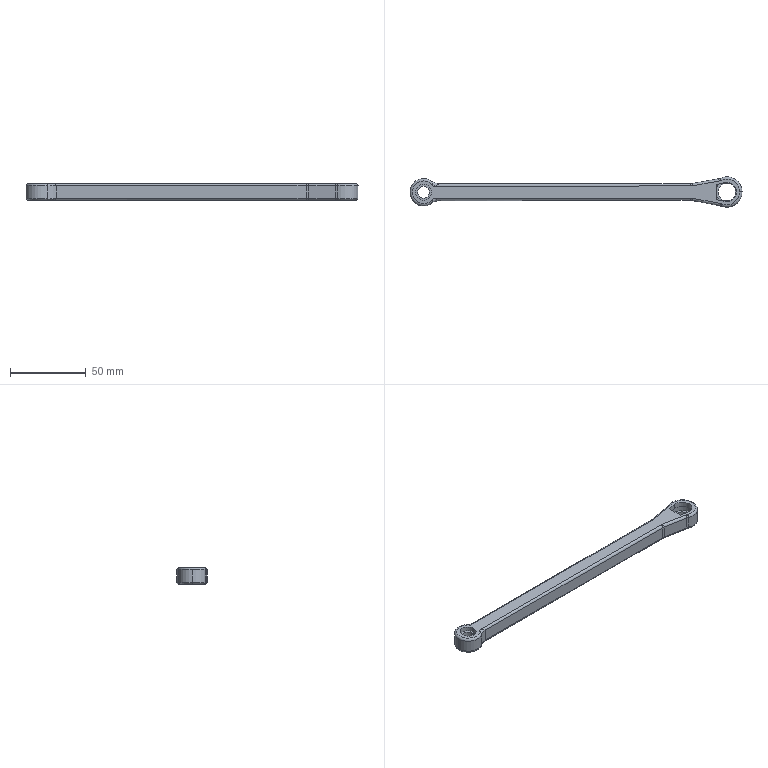Part | SolidWorks | features ICE 10, Fillet 2, Extrusion 1 | 1 solid | 63 faces | box 219 x 20 x 11 mm | volume 26143 mm3 | cylinder 29 | plane 16 | spline 12 | torus 6 | commonest cylinder face diameters 3 x8 20 x7 10.4 x4 7.7 x2 11.5 x2 12.6 x2